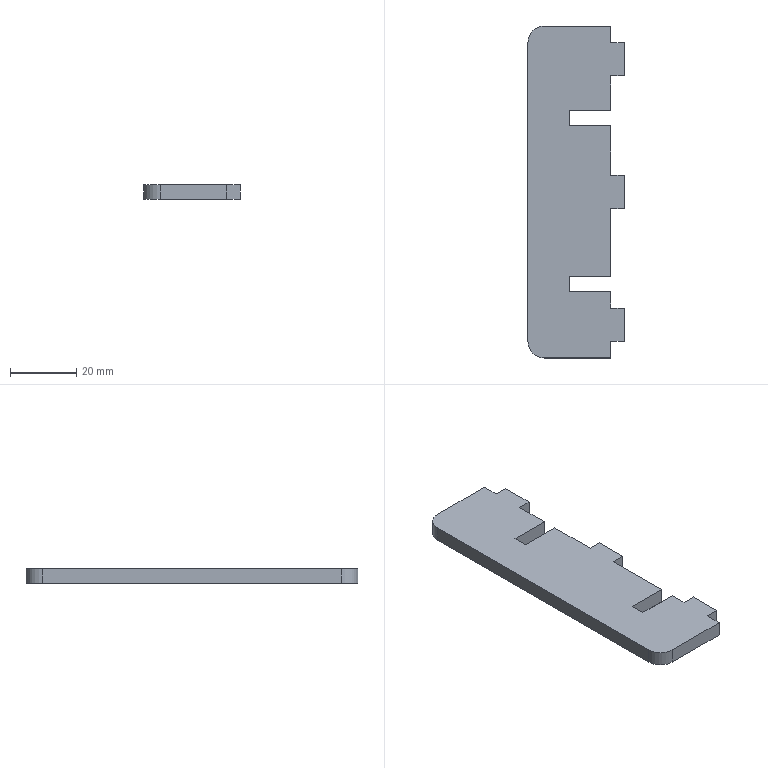Part | SolidWorks | features FlatPattern 1, SMBaseFlange 1, SheetMetal 1 | 1 solid | 28 faces | box 29 x 100 x 4.5 mm | volume 11235 mm3 | plane 26 | cylinder 2 | commonest cylinder face diameters 10 x2
STEP:
#1=CARTESIAN_POINT('',(115.747,10.575,0.));
#2=VERTEX_POINT('',#1);
#3=CARTESIAN_POINT('',(115.747,15.575,0.));
#4=VERTEX_POINT('',#3);
#5=CARTESIAN_POINT('',(115.747,15.575,0.));
#6=DIRECTION('',(0.,1.,0.));
#7=VECTOR('',#6,1000.);
#8=LINE('',#5,#7);
#9=EDGE_CURVE('',#2,#4,#8,.T.);
#10=ORIENTED_EDGE('',*,*,#9,.F.);
#11=CARTESIAN_POINT('',(115.747,10.575,-4.5));
#12=VERTEX_POINT('',#11);
#13=CARTESIAN_POINT('',(115.747,10.575,-4.5));
#14=DIRECTION('',(0.,0.,1.));
#15=VECTOR('',#14,1000.);
#16=LINE('',#13,#15);
#17=EDGE_CURVE('',#12,#2,#16,.T.);
#18=ORIENTED_EDGE('',*,*,#17,.F.);
#19=CARTESIAN_POINT('',(115.747,15.575,-4.5));
#20=VERTEX_POINT('',#19);
#21=CARTESIAN_POINT('',(115.747,15.575,-4.5));
#22=DIRECTION('',(0.,1.,0.));
#23=VECTOR('',#22,1000.);
#24=LINE('',#21,#23);
#25=EDGE_CURVE('',#12,#20,#24,.T.);
#26=ORIENTED_EDGE('',*,*,#25,.T.);
#27=CARTESIAN_POINT('',(115.747,15.575,-4.5));
#28=DIRECTION('',(0.,0.,1.));
#29=VECTOR('',#28,1000.);
#30=LINE('',#27,#29);
#31=EDGE_CURVE('',#20,#4,#30,.T.);
#32=ORIENTED_EDGE('',*,*,#31,.T.);
#33=EDGE_LOOP('',(#10,#18,#26,#32));
#34=FACE_OUTER_BOUND('',#33,.T.);
#35=CARTESIAN_POINT('',(115.747,15.575,-4.5));
#36=DIRECTION('',(1.,0.,0.));
#37=DIRECTION('',(0.,0.,-1.));
#38=AXIS2_PLACEMENT_3D('',#35,#36,#37);
#39=PLANE('',#38);
#40=ADVANCED_FACE('',(#34),#39,.T.);
#41=CARTESIAN_POINT('',(119.747,10.575,0.));
#42=VERTEX_POINT('',#41);
#43=CARTESIAN_POINT('',(115.747,10.575,0.));
#44=DIRECTION('',(-1.,0.,0.));
#45=VECTOR('',#44,1000.);
#46=LINE('',#43,#45);
#47=EDGE_CURVE('',#42,#2,#46,.T.);
#48=ORIENTED_EDGE('',*,*,#47,.F.);
#49=CARTESIAN_POINT('',(119.747,10.575,-4.5));
#50=VERTEX_POINT('',#49);
#51=CARTESIAN_POINT('',(119.747,10.575,-4.5));
#52=DIRECTION('',(0.,0.,1.));
#53=VECTOR('',#52,1000.);
#54=LINE('',#51,#53);
#55=EDGE_CURVE('',#50,#42,#54,.T.);
#56=ORIENTED_EDGE('',*,*,#55,.F.);
#57=CARTESIAN_POINT('',(115.747,10.575,-4.5));
#58=DIRECTION('',(-1.,0.,0.));
#59=VECTOR('',#58,1000.);
#60=LINE('',#57,#59);
#61=EDGE_CURVE('',#50,#12,#60,.T.);
#62=ORIENTED_EDGE('',*,*,#61,.T.);
#63=ORIENTED_EDGE('',*,*,#17,.T.);
#64=EDGE_LOOP('',(#48,#56,#62,#63));
#65=FACE_OUTER_BOUND('',#64,.T.);
#66=CARTESIAN_POINT('',(115.747,10.575,-4.5));
#67=DIRECTION('',(0.,1.,0.));
#68=DIRECTION('',(0.,0.,1.));
#69=AXIS2_PLACEMENT_3D('',#66,#67,#68);
#70=PLANE('',#69);
#71=ADVANCED_FACE('',(#65),#70,.T.);
#72=CARTESIAN_POINT('',(119.747,0.5749,0.));
#73=VERTEX_POINT('',#72);
#74=CARTESIAN_POINT('',(119.747,10.575,0.));
#75=DIRECTION('',(0.,1.,0.));
#76=VECTOR('',#75,1000.);
#77=LINE('',#74,#76);
#78=EDGE_CURVE('',#73,#42,#77,.T.);
#79=ORIENTED_EDGE('',*,*,#78,.F.);
#80=CARTESIAN_POINT('',(119.747,0.5749,-4.5));
#81=VERTEX_POINT('',#80);
#82=CARTESIAN_POINT('',(119.747,0.5749,-4.5));
#83=DIRECTION('',(0.,0.,1.));
#84=VECTOR('',#83,1000.);
#85=LINE('',#82,#84);
#86=EDGE_CURVE('',#81,#73,#85,.T.);
#87=ORIENTED_EDGE('',*,*,#86,.F.);
#88=CARTESIAN_POINT('',(119.747,10.575,-4.5));
#89=DIRECTION('',(0.,1.,0.));
#90=VECTOR('',#89,1000.);
#91=LINE('',#88,#90);
#92=EDGE_CURVE('',#81,#50,#91,.T.);
#93=ORIENTED_EDGE('',*,*,#92,.T.);
#94=ORIENTED_EDGE('',*,*,#55,.T.);
#95=EDGE_LOOP('',(#79,#87,#93,#94));
#96=FACE_OUTER_BOUND('',#95,.T.);
#97=CARTESIAN_POINT('',(119.747,10.575,-4.5));
#98=DIRECTION('',(1.,0.,0.));
#99=DIRECTION('',(0.,0.,-1.));
#100=AXIS2_PLACEMENT_3D('',#97,#98,#99);
#101=PLANE('',#100);
#102=ADVANCED_FACE('',(#96),#101,.T.);
#103=CARTESIAN_POINT('',(115.747,0.5749,0.));
#104=VERTEX_POINT('',#103);
#105=CARTESIAN_POINT('',(119.747,0.5749,0.));
#106=DIRECTION('',(1.,0.,0.));
#107=VECTOR('',#106,1000.);
#108=LINE('',#105,#107);
#109=EDGE_CURVE('',#104,#73,#108,.T.);
#110=ORIENTED_EDGE('',*,*,#109,.F.);
#111=CARTESIAN_POINT('',(115.747,0.5749,-4.5));
#112=VERTEX_POINT('',#111);
#113=CARTESIAN_POINT('',(115.747,0.5749,-4.5));
#114=DIRECTION('',(0.,0.,1.));
#115=VECTOR('',#114,1000.);
#116=LINE('',#113,#115);
#117=EDGE_CURVE('',#112,#104,#116,.T.);
#118=ORIENTED_EDGE('',*,*,#117,.F.);
#119=CARTESIAN_POINT('',(119.747,0.5749,-4.5));
#120=DIRECTION('',(1.,0.,0.));
#121=VECTOR('',#120,1000.);
#122=LINE('',#119,#121);
#123=EDGE_CURVE('',#112,#81,#122,.T.);
#124=ORIENTED_EDGE('',*,*,#123,.T.);
#125=ORIENTED_EDGE('',*,*,#86,.T.);
#126=EDGE_LOOP('',(#110,#118,#124,#125));
#127=FACE_OUTER_BOUND('',#126,.T.);
#128=CARTESIAN_POINT('',(119.747,0.5749,-4.5));
#129=DIRECTION('',(0.,-1.,0.));
#130=DIRECTION('',(1.,0.,0.));
#131=AXIS2_PLACEMENT_3D('',#128,#129,#130);
#132=PLANE('',#131);
#133=ADVANCED_FACE('',(#127),#132,.T.);
#134=CARTESIAN_POINT('',(115.747,-9.925,0.));
#135=VERTEX_POINT('',#134);
#136=CARTESIAN_POINT('',(115.747,0.5749,0.));
#137=DIRECTION('',(0.,1.,0.));
#138=VECTOR('',#137,1000.);
#139=LINE('',#136,#138);
#140=EDGE_CURVE('',#135,#104,#139,.T.);
#141=ORIENTED_EDGE('',*,*,#140,.F.);
#142=CARTESIAN_POINT('',(115.747,-9.925,-4.5));
#143=VERTEX_POINT('',#142);
#144=CARTESIAN_POINT('',(115.747,-9.925,-4.5));
#145=DIRECTION('',(0.,0.,1.));
#146=VECTOR('',#145,1000.);
#147=LINE('',#144,#146);
#148=EDGE_CURVE('',#143,#135,#147,.T.);
#149=ORIENTED_EDGE('',*,*,#148,.F.);
#150=CARTESIAN_POINT('',(115.747,0.5749,-4.5));
#151=DIRECTION('',(0.,1.,0.));
#152=VECTOR('',#151,1000.);
#153=LINE('',#150,#152);
#154=EDGE_CURVE('',#143,#112,#153,.T.);
#155=ORIENTED_EDGE('',*,*,#154,.T.);
#156=ORIENTED_EDGE('',*,*,#117,.T.);
#157=EDGE_LOOP('',(#141,#149,#155,#156));
#158=FACE_OUTER_BOUND('',#157,.T.);
#159=CARTESIAN_POINT('',(115.747,0.5749,-4.5));
#160=DIRECTION('',(1.,0.,0.));
#161=DIRECTION('',(0.,1.,0.));
#162=AXIS2_PLACEMENT_3D('',#159,#160,#161);
#163=PLANE('',#162);
#164=ADVANCED_FACE('',(#158),#163,.T.);
#165=CARTESIAN_POINT('',(103.247,-9.925,0.));
#166=VERTEX_POINT('',#165);
#167=CARTESIAN_POINT('',(115.747,-9.925,0.));
#168=DIRECTION('',(1.,0.,0.));
#169=VECTOR('',#168,1000.);
#170=LINE('',#167,#169);
#171=EDGE_CURVE('',#166,#135,#170,.T.);
#172=ORIENTED_EDGE('',*,*,#171,.F.);
#173=CARTESIAN_POINT('',(103.247,-9.925,-4.5));
#174=VERTEX_POINT('',#173);
#175=CARTESIAN_POINT('',(103.247,-9.925,-4.5));
#176=DIRECTION('',(0.,0.,1.));
#177=VECTOR('',#176,1000.);
#178=LINE('',#175,#177);
#179=EDGE_CURVE('',#174,#166,#178,.T.);
#180=ORIENTED_EDGE('',*,*,#179,.F.);
#181=CARTESIAN_POINT('',(115.747,-9.925,-4.5));
#182=DIRECTION('',(1.,0.,0.));
#183=VECTOR('',#182,1000.);
#184=LINE('',#181,#183);
#185=EDGE_CURVE('',#174,#143,#184,.T.);
#186=ORIENTED_EDGE('',*,*,#185,.T.);
#187=ORIENTED_EDGE('',*,*,#148,.T.);
#188=EDGE_LOOP('',(#172,#180,#186,#187));
#189=FACE_OUTER_BOUND('',#188,.T.);
#190=CARTESIAN_POINT('',(115.747,-9.925,-4.5));
#191=DIRECTION('',(0.,-1.,0.));
#192=DIRECTION('',(0.,0.,-1.));
#193=AXIS2_PLACEMENT_3D('',#190,#191,#192);
#194=PLANE('',#193);
#195=ADVANCED_FACE('',(#189),#194,.T.);
#196=CARTESIAN_POINT('',(103.247,-14.425,0.));
#197=VERTEX_POINT('',#196);
#198=CARTESIAN_POINT('',(103.247,-9.925,0.));
#199=DIRECTION('',(0.,1.,0.));
#200=VECTOR('',#199,1000.);
#201=LINE('',#198,#200);
#202=EDGE_CURVE('',#197,#166,#201,.T.);
#203=ORIENTED_EDGE('',*,*,#202,.F.);
#204=CARTESIAN_POINT('',(103.247,-14.425,-4.5));
#205=VERTEX_POINT('',#204);
#206=CARTESIAN_POINT('',(103.247,-14.425,-4.5));
#207=DIRECTION('',(0.,0.,1.));
#208=VECTOR('',#207,1000.);
#209=LINE('',#206,#208);
#210=EDGE_CURVE('',#205,#197,#209,.T.);
#211=ORIENTED_EDGE('',*,*,#210,.F.);
#212=CARTESIAN_POINT('',(103.247,-9.925,-4.5));
#213=DIRECTION('',(0.,1.,0.));
#214=VECTOR('',#213,1000.);
#215=LINE('',#212,#214);
#216=EDGE_CURVE('',#205,#174,#215,.T.);
#217=ORIENTED_EDGE('',*,*,#216,.T.);
#218=ORIENTED_EDGE('',*,*,#179,.T.);
#219=EDGE_LOOP('',(#203,#211,#217,#218));
#220=FACE_OUTER_BOUND('',#219,.T.);
#221=CARTESIAN_POINT('',(103.247,-9.925,-4.5));
#222=DIRECTION('',(1.,0.,0.));
#223=DIRECTION('',(0.,0.,-1.));
#224=AXIS2_PLACEMENT_3D('',#221,#222,#223);
#225=PLANE('',#224);
#226=ADVANCED_FACE('',(#220),#225,.T.);
#227=CARTESIAN_POINT('',(115.747,-14.425,0.));
#228=VERTEX_POINT('',#227);
#229=CARTESIAN_POINT('',(103.247,-14.425,0.));
#230=DIRECTION('',(-1.,0.,0.));
#231=VECTOR('',#230,1000.);
#232=LINE('',#229,#231);
#233=EDGE_CURVE('',#228,#197,#232,.T.);
#234=ORIENTED_EDGE('',*,*,#233,.F.);
#235=CARTESIAN_POINT('',(115.747,-14.425,-4.5));
#236=VERTEX_POINT('',#235);
#237=CARTESIAN_POINT('',(115.747,-14.425,-4.5));
#238=DIRECTION('',(0.,0.,1.));
#239=VECTOR('',#238,1000.);
#240=LINE('',#237,#239);
#241=EDGE_CURVE('',#236,#228,#240,.T.);
#242=ORIENTED_EDGE('',*,*,#241,.F.);
#243=CARTESIAN_POINT('',(103.247,-14.425,-4.5));
#244=DIRECTION('',(-1.,0.,0.));
#245=VECTOR('',#244,1000.);
#246=LINE('',#243,#245);
#247=EDGE_CURVE('',#236,#205,#246,.T.);
#248=ORIENTED_EDGE('',*,*,#247,.T.);
#249=ORIENTED_EDGE('',*,*,#210,.T.);
#250=EDGE_LOOP('',(#234,#242,#248,#249));
#251=FACE_OUTER_BOUND('',#250,.T.);
#252=CARTESIAN_POINT('',(103.247,-14.425,-4.5));
#253=DIRECTION('',(0.,1.,0.));
#254=DIRECTION('',(0.,0.,1.));
#255=AXIS2_PLACEMENT_3D('',#252,#253,#254);
#256=PLANE('',#255);
#257=ADVANCED_FACE('',(#251),#256,.T.);
#258=CARTESIAN_POINT('',(115.747,-29.425,0.));
#259=VERTEX_POINT('',#258);
#260=CARTESIAN_POINT('',(115.747,-14.425,0.));
#261=DIRECTION('',(0.,1.,0.));
#262=VECTOR('',#261,1000.);
#263=LINE('',#260,#262);
#264=EDGE_CURVE('',#259,#228,#263,.T.);
#265=ORIENTED_EDGE('',*,*,#264,.F.);
#266=CARTESIAN_POINT('',(115.747,-29.425,-4.5));
#267=VERTEX_POINT('',#266);
#268=CARTESIAN_POINT('',(115.747,-29.425,-4.5));
#269=DIRECTION('',(0.,0.,1.));
#270=VECTOR('',#269,1000.);
#271=LINE('',#268,#270);
#272=EDGE_CURVE('',#267,#259,#271,.T.);
#273=ORIENTED_EDGE('',*,*,#272,.F.);
#274=CARTESIAN_POINT('',(115.747,-14.425,-4.5));
#275=DIRECTION('',(0.,1.,0.));
#276=VECTOR('',#275,1000.);
#277=LINE('',#274,#276);
#278=EDGE_CURVE('',#267,#236,#277,.T.);
#279=ORIENTED_EDGE('',*,*,#278,.T.);
#280=ORIENTED_EDGE('',*,*,#241,.T.);
#281=EDGE_LOOP('',(#265,#273,#279,#280));
#282=FACE_OUTER_BOUND('',#281,.T.);
#283=CARTESIAN_POINT('',(115.747,-14.425,-4.5));
#284=DIRECTION('',(1.,0.,0.));
#285=DIRECTION('',(0.,1.,0.));
#286=AXIS2_PLACEMENT_3D('',#283,#284,#285);
#287=PLANE('',#286);
#288=ADVANCED_FACE('',(#282),#287,.T.);
#289=CARTESIAN_POINT('',(119.747,-29.425,0.));
#290=VERTEX_POINT('',#289);
#291=CARTESIAN_POINT('',(115.747,-29.425,0.));
#292=DIRECTION('',(-1.,0.,0.));
#293=VECTOR('',#292,1000.);
#294=LINE('',#291,#293);
#295=EDGE_CURVE('',#290,#259,#294,.T.);
#296=ORIENTED_EDGE('',*,*,#295,.F.);
#297=CARTESIAN_POINT('',(119.747,-29.425,-4.5));
#298=VERTEX_POINT('',#297);
#299=CARTESIAN_POINT('',(119.747,-29.425,-4.5));
#300=DIRECTION('',(0.,0.,1.));
#301=VECTOR('',#300,1000.);
#302=LINE('',#299,#301);
#303=EDGE_CURVE('',#298,#290,#302,.T.);
#304=ORIENTED_EDGE('',*,*,#303,.F.);
#305=CARTESIAN_POINT('',(115.747,-29.425,-4.5));
#306=DIRECTION('',(-1.,0.,0.));
#307=VECTOR('',#306,1000.);
#308=LINE('',#305,#307);
#309=EDGE_CURVE('',#298,#267,#308,.T.);
#310=ORIENTED_EDGE('',*,*,#309,.T.);
#311=ORIENTED_EDGE('',*,*,#272,.T.);
#312=EDGE_LOOP('',(#296,#304,#310,#311));
#313=FACE_OUTER_BOUND('',#312,.T.);
#314=CARTESIAN_POINT('',(115.747,-29.425,-4.5));
#315=DIRECTION('',(0.,1.,0.));
#316=DIRECTION('',(0.,0.,1.));
#317=AXIS2_PLACEMENT_3D('',#314,#315,#316);
#318=PLANE('',#317);
#319=ADVANCED_FACE('',(#313),#318,.T.);
#320=CARTESIAN_POINT('',(119.747,-39.425,0.));
#321=VERTEX_POINT('',#320);
#322=CARTESIAN_POINT('',(119.747,-29.425,0.));
#323=DIRECTION('',(0.,1.,0.));
#324=VECTOR('',#323,1000.);
#325=LINE('',#322,#324);
#326=EDGE_CURVE('',#321,#290,#325,.T.);
#327=ORIENTED_EDGE('',*,*,#326,.F.);
#328=CARTESIAN_POINT('',(119.747,-39.425,-4.5));
#329=VERTEX_POINT('',#328);
#330=CARTESIAN_POINT('',(119.747,-39.425,-4.5));
#331=DIRECTION('',(0.,0.,1.));
#332=VECTOR('',#331,1000.);
#333=LINE('',#330,#332);
#334=EDGE_CURVE('',#329,#321,#333,.T.);
#335=ORIENTED_EDGE('',*,*,#334,.F.);
#336=CARTESIAN_POINT('',(119.747,-29.425,-4.5));
#337=DIRECTION('',(0.,1.,0.));
#338=VECTOR('',#337,1000.);
#339=LINE('',#336,#338);
#340=EDGE_CURVE('',#329,#298,#339,.T.);
#341=ORIENTED_EDGE('',*,*,#340,.T.);
#342=ORIENTED_EDGE('',*,*,#303,.T.);
#343=EDGE_LOOP('',(#327,#335,#341,#342));
#344=FACE_OUTER_BOUND('',#343,.T.);
#345=CARTESIAN_POINT('',(119.747,-29.425,-4.5));
#346=DIRECTION('',(1.,0.,0.));
#347=DIRECTION('',(0.,0.,-1.));
#348=AXIS2_PLACEMENT_3D('',#345,#346,#347);
#349=PLANE('',#348);
#350=ADVANCED_FACE('',(#344),#349,.T.);
#351=CARTESIAN_POINT('',(115.747,-39.425,0.));
#352=VERTEX_POINT('',#351);
#353=CARTESIAN_POINT('',(119.747,-39.425,0.));
#354=DIRECTION('',(1.,0.,0.));
#355=VECTOR('',#354,1000.);
#356=LINE('',#353,#355);
#357=EDGE_CURVE('',#352,#321,#356,.T.);
#358=ORIENTED_EDGE('',*,*,#357,.F.);
#359=CARTESIAN_POINT('',(115.747,-39.425,-4.5));
#360=VERTEX_POINT('',#359);
#361=CARTESIAN_POINT('',(115.747,-39.425,-4.5));
#362=DIRECTION('',(0.,0.,1.));
#363=VECTOR('',#362,1000.);
#364=LINE('',#361,#363);
#365=EDGE_CURVE('',#360,#352,#364,.T.);
#366=ORIENTED_EDGE('',*,*,#365,.F.);
#367=CARTESIAN_POINT('',(119.747,-39.425,-4.5));
#368=DIRECTION('',(1.,0.,0.));
#369=VECTOR('',#368,1000.);
#370=LINE('',#367,#369);
#371=EDGE_CURVE('',#360,#329,#370,.T.);
#372=ORIENTED_EDGE('',*,*,#371,.T.);
#373=ORIENTED_EDGE('',*,*,#334,.T.);
#374=EDGE_LOOP('',(#358,#366,#372,#373));
#375=FACE_OUTER_BOUND('',#374,.T.);
#376=CARTESIAN_POINT('',(119.747,-39.425,-4.5));
#377=DIRECTION('',(0.,-1.,0.));
#378=DIRECTION('',(0.,0.,-1.));
#379=AXIS2_PLACEMENT_3D('',#376,#377,#378);
#380=PLANE('',#379);
#381=ADVANCED_FACE('',(#375),#380,.T.);
#382=CARTESIAN_POINT('',(115.747,-59.925,0.));
#383=VERTEX_POINT('',#382);
#384=CARTESIAN_POINT('',(115.747,-39.425,0.));
#385=DIRECTION('',(0.,1.,0.));
#386=VECTOR('',#385,1000.);
#387=LINE('',#384,#386);
#388=EDGE_CURVE('',#383,#352,#387,.T.);
#389=ORIENTED_EDGE('',*,*,#388,.F.);
#390=CARTESIAN_POINT('',(115.747,-59.925,-4.5));
#391=VERTEX_POINT('',#390);
#392=CARTESIAN_POINT('',(115.747,-59.925,-4.5));
#393=DIRECTION('',(0.,0.,1.));
#394=VECTOR('',#393,1000.);
#395=LINE('',#392,#394);
#396=EDGE_CURVE('',#391,#383,#395,.T.);
#397=ORIENTED_EDGE('',*,*,#396,.F.);
#398=CARTESIAN_POINT('',(115.747,-39.425,-4.5));
#399=DIRECTION('',(0.,1.,0.));
#400=VECTOR('',#399,1000.);
#401=LINE('',#398,#400);
#402=EDGE_CURVE('',#391,#360,#401,.T.);
#403=ORIENTED_EDGE('',*,*,#402,.T.);
#404=ORIENTED_EDGE('',*,*,#365,.T.);
#405=EDGE_LOOP('',(#389,#397,#403,#404));
#406=FACE_OUTER_BOUND('',#405,.T.);
#407=CARTESIAN_POINT('',(115.747,-39.425,-4.5));
#408=DIRECTION('',(1.,0.,0.));
#409=DIRECTION('',(0.,1.,0.));
#410=AXIS2_PLACEMENT_3D('',#407,#408,#409);
#411=PLANE('',#410);
#412=ADVANCED_FACE('',(#406),#411,.T.);
#413=CARTESIAN_POINT('',(103.247,-59.925,0.));
#414=VERTEX_POINT('',#413);
#415=CARTESIAN_POINT('',(115.747,-59.925,0.));
#416=DIRECTION('',(1.,0.,0.));
#417=VECTOR('',#416,1000.);
#418=LINE('',#415,#417);
#419=EDGE_CURVE('',#414,#383,#418,.T.);
#420=ORIENTED_EDGE('',*,*,#419,.F.);
#421=CARTESIAN_POINT('',(103.247,-59.925,-4.5));
#422=VERTEX_POINT('',#421);
#423=CARTESIAN_POINT('',(103.247,-59.925,-4.5));
#424=DIRECTION('',(0.,0.,1.));
#425=VECTOR('',#424,1000.);
#426=LINE('',#423,#425);
#427=EDGE_CURVE('',#422,#414,#426,.T.);
#428=ORIENTED_EDGE('',*,*,#427,.F.);
#429=CARTESIAN_POINT('',(115.747,-59.925,-4.5));
#430=DIRECTION('',(1.,0.,0.));
#431=VECTOR('',#430,1000.);
#432=LINE('',#429,#431);
#433=EDGE_CURVE('',#422,#391,#432,.T.);
#434=ORIENTED_EDGE('',*,*,#433,.T.);
#435=ORIENTED_EDGE('',*,*,#396,.T.);
#436=EDGE_LOOP('',(#420,#428,#434,#435));
#437=FACE_OUTER_BOUND('',#436,.T.);
#438=CARTESIAN_POINT('',(115.747,-59.925,-4.5));
#439=DIRECTION('',(0.,-1.,0.));
#440=DIRECTION('',(0.,0.,-1.));
#441=AXIS2_PLACEMENT_3D('',#438,#439,#440);
#442=PLANE('',#441);
#443=ADVANCED_FACE('',(#437),#442,.T.);
#444=CARTESIAN_POINT('',(103.247,-64.425,0.));
#445=VERTEX_POINT('',#444);
#446=CARTESIAN_POINT('',(103.247,-59.925,0.));
#447=DIRECTION('',(0.,1.,0.));
#448=VECTOR('',#447,1000.);
#449=LINE('',#446,#448);
#450=EDGE_CURVE('',#445,#414,#449,.T.);
#451=ORIENTED_EDGE('',*,*,#450,.F.);
#452=CARTESIAN_POINT('',(103.247,-64.425,-4.5));
#453=VERTEX_POINT('',#452);
#454=CARTESIAN_POINT('',(103.247,-64.425,-4.5));
#455=DIRECTION('',(0.,0.,1.));
#456=VECTOR('',#455,1000.);
#457=LINE('',#454,#456);
#458=EDGE_CURVE('',#453,#445,#457,.T.);
#459=ORIENTED_EDGE('',*,*,#458,.F.);
#460=CARTESIAN_POINT('',(103.247,-59.925,-4.5));
#461=DIRECTION('',(0.,1.,0.));
#462=VECTOR('',#461,1000.);
#463=LINE('',#460,#462);
#464=EDGE_CURVE('',#453,#422,#463,.T.);
#465=ORIENTED_EDGE('',*,*,#464,.T.);
#466=ORIENTED_EDGE('',*,*,#427,.T.);
#467=EDGE_LOOP('',(#451,#459,#465,#466));
#468=FACE_OUTER_BOUND('',#467,.T.);
#469=CARTESIAN_POINT('',(103.247,-59.925,-4.5));
#470=DIRECTION('',(1.,0.,0.));
#471=DIRECTION('',(0.,0.,-1.));
#472=AXIS2_PLACEMENT_3D('',#469,#470,#471);
#473=PLANE('',#472);
#474=ADVANCED_FACE('',(#468),#473,.T.);
#475=CARTESIAN_POINT('',(115.747,-64.425,0.));
#476=VERTEX_POINT('',#475);
#477=CARTESIAN_POINT('',(103.247,-64.425,0.));
#478=DIRECTION('',(-1.,0.,0.));
#479=VECTOR('',#478,1000.);
#480=LINE('',#477,#479);
#481=EDGE_CURVE('',#476,#445,#480,.T.);
#482=ORIENTED_EDGE('',*,*,#481,.F.);
#483=CARTESIAN_POINT('',(115.747,-64.425,-4.5));
#484=VERTEX_POINT('',#483);
#485=CARTESIAN_POINT('',(115.747,-64.425,-4.5));
#486=DIRECTION('',(0.,0.,1.));
#487=VECTOR('',#486,1000.);
#488=LINE('',#485,#487);
#489=EDGE_CURVE('',#484,#476,#488,.T.);
#490=ORIENTED_EDGE('',*,*,#489,.F.);
#491=CARTESIAN_POINT('',(103.247,-64.425,-4.5));
#492=DIRECTION('',(-1.,0.,0.));
#493=VECTOR('',#492,1000.);
#494=LINE('',#491,#493);
#495=EDGE_CURVE('',#484,#453,#494,.T.);
#496=ORIENTED_EDGE('',*,*,#495,.T.);
#497=ORIENTED_EDGE('',*,*,#458,.T.);
#498=EDGE_LOOP('',(#482,#490,#496,#497));
#499=FACE_OUTER_BOUND('',#498,.T.);
#500=CARTESIAN_POINT('',(103.247,-64.425,-4.5));
#501=DIRECTION('',(0.,1.,0.));
#502=DIRECTION('',(0.,0.,1.));
#503=AXIS2_PLACEMENT_3D('',#500,#501,#502);
#504=PLANE('',#503);
#505=ADVANCED_FACE('',(#499),#504,.T.);
#506=CARTESIAN_POINT('',(115.747,-69.425,0.));
#507=VERTEX_POINT('',#506);
#508=CARTESIAN_POINT('',(115.747,-64.425,0.));
#509=DIRECTION('',(0.,1.,0.));
#510=VECTOR('',#509,1000.);
#511=LINE('',#508,#510);
#512=EDGE_CURVE('',#507,#476,#511,.T.);
#513=ORIENTED_EDGE('',*,*,#512,.F.);
#514=CARTESIAN_POINT('',(115.747,-69.425,-4.5));
#515=VERTEX_POINT('',#514);
#516=CARTESIAN_POINT('',(115.747,-69.425,-4.5));
#517=DIRECTION('',(0.,0.,1.));
#518=VECTOR('',#517,1000.);
#519=LINE('',#516,#518);
#520=EDGE_CURVE('',#515,#507,#519,.T.);
#521=ORIENTED_EDGE('',*,*,#520,.F.);
#522=CARTESIAN_POINT('',(115.747,-64.425,-4.5));
#523=DIRECTION('',(0.,1.,0.));
#524=VECTOR('',#523,1000.);
#525=LINE('',#522,#524);
#526=EDGE_CURVE('',#515,#484,#525,.T.);
#527=ORIENTED_EDGE('',*,*,#526,.T.);
#528=ORIENTED_EDGE('',*,*,#489,.T.);
#529=EDGE_LOOP('',(#513,#521,#527,#528));
#530=FACE_OUTER_BOUND('',#529,.T.);
#531=CARTESIAN_POINT('',(115.747,-64.425,-4.5));
#532=DIRECTION('',(1.,0.,0.));
#533=DIRECTION('',(0.,0.,-1.));
#534=AXIS2_PLACEMENT_3D('',#531,#532,#533);
#535=PLANE('',#534);
#536=ADVANCED_FACE('',(#530),#535,.T.);
#537=CARTESIAN_POINT('',(119.747,-69.425,0.));
#538=VERTEX_POINT('',#537);
#539=CARTESIAN_POINT('',(119.747,-69.425,0.));
#540=DIRECTION('',(-1.,0.,0.));
#541=VECTOR('',#540,1000.);
#542=LINE('',#539,#541);
#543=EDGE_CURVE('',#538,#507,#542,.T.);
#544=ORIENTED_EDGE('',*,*,#543,.F.);
#545=CARTESIAN_POINT('',(119.747,-69.425,-4.5));
#546=VERTEX_POINT('',#545);
#547=CARTESIAN_POINT('',(119.747,-69.425,-4.5));
#548=DIRECTION('',(0.,0.,1.));
#549=VECTOR('',#548,1000.);
#550=LINE('',#547,#549);
#551=EDGE_CURVE('',#546,#538,#550,.T.);
#552=ORIENTED_EDGE('',*,*,#551,.F.);
#553=CARTESIAN_POINT('',(119.747,-69.425,-4.5));
#554=DIRECTION('',(-1.,0.,0.));
#555=VECTOR('',#554,1000.);
#556=LINE('',#553,#555);
#557=EDGE_CURVE('',#546,#515,#556,.T.);
#558=ORIENTED_EDGE('',*,*,#557,.T.);
#559=ORIENTED_EDGE('',*,*,#520,.T.);
#560=EDGE_LOOP('',(#544,#552,#558,#559));
#561=FACE_OUTER_BOUND('',#560,.T.);
#562=CARTESIAN_POINT('',(119.747,-69.425,-4.5));
#563=DIRECTION('',(0.,1.,0.));
#564=DIRECTION('',(0.,0.,1.));
#565=AXIS2_PLACEMENT_3D('',#562,#563,#564);
#566=PLANE('',#565);
#567=ADVANCED_FACE('',(#561),#566,.T.);
#568=CARTESIAN_POINT('',(119.747,-79.425,0.));
#569=VERTEX_POINT('',#568);
#570=CARTESIAN_POINT('',(119.747,-79.425,0.));
#571=DIRECTION('',(0.,1.,0.));
#572=VECTOR('',#571,1000.);
#573=LINE('',#570,#572);
#574=EDGE_CURVE('',#569,#538,#573,.T.);
#575=ORIENTED_EDGE('',*,*,#574,.F.);
#576=CARTESIAN_POINT('',(119.747,-79.425,-4.5));
#577=VERTEX_POINT('',#576);
#578=CARTESIAN_POINT('',(119.747,-79.425,-4.5));
#579=DIRECTION('',(0.,0.,1.));
#580=VECTOR('',#579,1000.);
#581=LINE('',#578,#580);
#582=EDGE_CURVE('',#577,#569,#581,.T.);
#583=ORIENTED_EDGE('',*,*,#582,.F.);
#584=CARTESIAN_POINT('',(119.747,-79.425,-4.5));
#585=DIRECTION('',(0.,1.,0.));
#586=VECTOR('',#585,1000.);
#587=LINE('',#584,#586);
#588=EDGE_CURVE('',#577,#546,#587,.T.);
#589=ORIENTED_EDGE('',*,*,#588,.T.);
#590=ORIENTED_EDGE('',*,*,#551,.T.);
#591=EDGE_LOOP('',(#575,#583,#589,#590));
#592=FACE_OUTER_BOUND('',#591,.T.);
#593=CARTESIAN_POINT('',(119.747,-79.425,-4.5));
#594=DIRECTION('',(1.,0.,0.));
#595=DIRECTION('',(0.,0.,-1.));
#596=AXIS2_PLACEMENT_3D('',#593,#594,#595);
#597=PLANE('',#596);
#598=ADVANCED_FACE('',(#592),#597,.T.);
#599=CARTESIAN_POINT('',(115.747,-79.425,0.));
#600=VERTEX_POINT('',#599);
#601=CARTESIAN_POINT('',(115.747,-79.425,0.));
#602=DIRECTION('',(1.,0.,0.));
#603=VECTOR('',#602,1000.);
#604=LINE('',#601,#603);
#605=EDGE_CURVE('',#600,#569,#604,.T.);
#606=ORIENTED_EDGE('',*,*,#605,.F.);
#607=CARTESIAN_POINT('',(115.747,-79.425,-4.5));
#608=VERTEX_POINT('',#607);
#609=CARTESIAN_POINT('',(115.747,-79.425,-4.5));
#610=DIRECTION('',(0.,0.,1.));
#611=VECTOR('',#610,1000.);
#612=LINE('',#609,#611);
#613=EDGE_CURVE('',#608,#600,#612,.T.);
#614=ORIENTED_EDGE('',*,*,#613,.F.);
#615=CARTESIAN_POINT('',(115.747,-79.425,-4.5));
#616=DIRECTION('',(1.,0.,0.));
#617=VECTOR('',#616,1000.);
#618=LINE('',#615,#617);
#619=EDGE_CURVE('',#608,#577,#618,.T.);
#620=ORIENTED_EDGE('',*,*,#619,.T.);
#621=ORIENTED_EDGE('',*,*,#582,.T.);
#622=EDGE_LOOP('',(#606,#614,#620,#621));
#623=FACE_OUTER_BOUND('',#622,.T.);
#624=CARTESIAN_POINT('',(115.747,-79.425,-4.5));
#625=DIRECTION('',(0.,-1.,0.));
#626=DIRECTION('',(0.,0.,-1.));
#627=AXIS2_PLACEMENT_3D('',#624,#625,#626);
#628=PLANE('',#627);
#629=ADVANCED_FACE('',(#623),#628,.T.);
#630=CARTESIAN_POINT('',(115.747,-84.425,0.));
#631=VERTEX_POINT('',#630);
#632=CARTESIAN_POINT('',(115.747,-79.425,0.));
#633=DIRECTION('',(0.,1.,0.));
#634=VECTOR('',#633,1000.);
#635=LINE('',#632,#634);
#636=EDGE_CURVE('',#631,#600,#635,.T.);
#637=ORIENTED_EDGE('',*,*,#636,.F.);
#638=CARTESIAN_POINT('',(115.747,-84.425,-4.5));
#639=VERTEX_POINT('',#638);
#640=CARTESIAN_POINT('',(115.747,-84.425,-4.5));
#641=DIRECTION('',(0.,0.,1.));
#642=VECTOR('',#641,1000.);
#643=LINE('',#640,#642);
#644=EDGE_CURVE('',#639,#631,#643,.T.);
#645=ORIENTED_EDGE('',*,*,#644,.F.);
#646=CARTESIAN_POINT('',(115.747,-79.425,-4.5));
#647=DIRECTION('',(0.,1.,0.));
#648=VECTOR('',#647,1000.);
#649=LINE('',#646,#648);
#650=EDGE_CURVE('',#639,#608,#649,.T.);
#651=ORIENTED_EDGE('',*,*,#650,.T.);
#652=ORIENTED_EDGE('',*,*,#613,.T.);
#653=EDGE_LOOP('',(#637,#645,#651,#652));
#654=FACE_OUTER_BOUND('',#653,.T.);
#655=CARTESIAN_POINT('',(115.747,-79.425,-4.5));
#656=DIRECTION('',(1.,0.,0.));
#657=DIRECTION('',(0.,0.,-1.));
#658=AXIS2_PLACEMENT_3D('',#655,#656,#657);
#659=PLANE('',#658);
#660=ADVANCED_FACE('',(#654),#659,.T.);
#661=CARTESIAN_POINT('',(95.747,-84.425,0.));
#662=VERTEX_POINT('',#661);
#663=CARTESIAN_POINT('',(115.747,-84.425,0.));
#664=DIRECTION('',(1.,0.,0.));
#665=VECTOR('',#664,1000.);
#666=LINE('',#663,#665);
#667=EDGE_CURVE('',#662,#631,#666,.T.);
#668=ORIENTED_EDGE('',*,*,#667,.F.);
#669=CARTESIAN_POINT('',(95.747,-84.425,-4.5));
#670=VERTEX_POINT('',#669);
#671=CARTESIAN_POINT('',(95.747,-84.425,-4.5));
#672=DIRECTION('',(0.,0.,1.));
#673=VECTOR('',#672,1000.);
#674=LINE('',#671,#673);
#675=EDGE_CURVE('',#670,#662,#674,.T.);
#676=ORIENTED_EDGE('',*,*,#675,.F.);
#677=CARTESIAN_POINT('',(115.747,-84.425,-4.5));
#678=DIRECTION('',(1.,0.,0.));
#679=VECTOR('',#678,1000.);
#680=LINE('',#677,#679);
#681=EDGE_CURVE('',#670,#639,#680,.T.);
#682=ORIENTED_EDGE('',*,*,#681,.T.);
#683=ORIENTED_EDGE('',*,*,#644,.T.);
#684=EDGE_LOOP('',(#668,#676,#682,#683));
#685=FACE_OUTER_BOUND('',#684,.T.);
#686=CARTESIAN_POINT('',(115.747,-84.425,-4.5));
#687=DIRECTION('',(0.,-1.,0.));
#688=DIRECTION('',(0.,0.,-1.));
#689=AXIS2_PLACEMENT_3D('',#686,#687,#688);
#690=PLANE('',#689);
#691=ADVANCED_FACE('',(#685),#690,.T.);
#692=CARTESIAN_POINT('',(90.747,-79.425,0.));
#693=VERTEX_POINT('',#692);
#694=CARTESIAN_POINT('',(95.747,-79.425,0.));
#695=DIRECTION('',(0.,0.,1.));
#696=DIRECTION('',(-1.,0.,0.));
#697=AXIS2_PLACEMENT_3D('',#694,#695,#696);
#698=CIRCLE('',#697,5.);
#699=EDGE_CURVE('',#693,#662,#698,.T.);
#700=ORIENTED_EDGE('',*,*,#699,.F.);
#701=CARTESIAN_POINT('',(90.747,-79.425,-4.5));
#702=VERTEX_POINT('',#701);
#703=CARTESIAN_POINT('',(90.747,-79.425,-4.5));
#704=DIRECTION('',(0.,0.,1.));
#705=VECTOR('',#704,1000.);
#706=LINE('',#703,#705);
#707=EDGE_CURVE('',#702,#693,#706,.T.);
#708=ORIENTED_EDGE('',*,*,#707,.F.);
#709=CARTESIAN_POINT('',(95.747,-79.425,-4.5));
#710=DIRECTION('',(0.,0.,1.));
#711=DIRECTION('',(-1.,0.,0.));
#712=AXIS2_PLACEMENT_3D('',#709,#710,#711);
#713=CIRCLE('',#712,5.);
#714=EDGE_CURVE('',#702,#670,#713,.T.);
#715=ORIENTED_EDGE('',*,*,#714,.T.);
#716=ORIENTED_EDGE('',*,*,#675,.T.);
#717=EDGE_LOOP('',(#700,#708,#715,#716));
#718=FACE_OUTER_BOUND('',#717,.T.);
#719=CARTESIAN_POINT('',(95.747,-79.425,-4.5));
#720=DIRECTION('',(0.,0.,1.));
#721=DIRECTION('',(1.,0.,0.));
#722=AXIS2_PLACEMENT_3D('',#719,#720,#721);
#723=CYLINDRICAL_SURFACE('',#722,5.);
#724=ADVANCED_FACE('',(#718),#723,.T.);
#725=CARTESIAN_POINT('',(90.747,10.575,0.));
#726=VERTEX_POINT('',#725);
#727=CARTESIAN_POINT('',(90.747,10.575,0.));
#728=DIRECTION('',(0.,-1.,0.));
#729=VECTOR('',#728,1000.);
#730=LINE('',#727,#729);
#731=EDGE_CURVE('',#726,#693,#730,.T.);
#732=ORIENTED_EDGE('',*,*,#731,.F.);
#733=CARTESIAN_POINT('',(90.747,10.575,-4.5));
#734=VERTEX_POINT('',#733);
#735=CARTESIAN_POINT('',(90.747,10.575,-4.5));
#736=DIRECTION('',(0.,0.,1.));
#737=VECTOR('',#736,1000.);
#738=LINE('',#735,#737);
#739=EDGE_CURVE('',#734,#726,#738,.T.);
#740=ORIENTED_EDGE('',*,*,#739,.F.);
#741=CARTESIAN_POINT('',(90.747,10.575,-4.5));
#742=DIRECTION('',(0.,-1.,0.));
#743=VECTOR('',#742,1000.);
#744=LINE('',#741,#743);
#745=EDGE_CURVE('',#734,#702,#744,.T.);
#746=ORIENTED_EDGE('',*,*,#745,.T.);
#747=ORIENTED_EDGE('',*,*,#707,.T.);
#748=EDGE_LOOP('',(#732,#740,#746,#747));
#749=FACE_OUTER_BOUND('',#748,.T.);
#750=CARTESIAN_POINT('',(90.747,10.575,-4.5));
#751=DIRECTION('',(-1.,0.,0.));
#752=DIRECTION('',(0.,-1.,0.));
#753=AXIS2_PLACEMENT_3D('',#750,#751,#752);
#754=PLANE('',#753);
#755=ADVANCED_FACE('',(#749),#754,.T.);
#756=CARTESIAN_POINT('',(95.747,15.575,0.));
#757=VERTEX_POINT('',#756);
#758=CARTESIAN_POINT('',(95.747,10.575,0.));
#759=DIRECTION('',(0.,0.,1.));
#760=DIRECTION('',(1.,0.,0.));
#761=AXIS2_PLACEMENT_3D('',#758,#759,#760);
#762=CIRCLE('',#761,5.);
#763=EDGE_CURVE('',#757,#726,#762,.T.);
#764=ORIENTED_EDGE('',*,*,#763,.F.);
#765=CARTESIAN_POINT('',(95.747,15.575,-4.5));
#766=VERTEX_POINT('',#765);
#767=CARTESIAN_POINT('',(95.747,15.575,-4.5));
#768=DIRECTION('',(0.,0.,1.));
#769=VECTOR('',#768,1000.);
#770=LINE('',#767,#769);
#771=EDGE_CURVE('',#766,#757,#770,.T.);
#772=ORIENTED_EDGE('',*,*,#771,.F.);
#773=CARTESIAN_POINT('',(95.747,10.575,-4.5));
#774=DIRECTION('',(0.,0.,1.));
#775=DIRECTION('',(1.,0.,0.));
#776=AXIS2_PLACEMENT_3D('',#773,#774,#775);
#777=CIRCLE('',#776,5.);
#778=EDGE_CURVE('',#766,#734,#777,.T.);
#779=ORIENTED_EDGE('',*,*,#778,.T.);
#780=ORIENTED_EDGE('',*,*,#739,.T.);
#781=EDGE_LOOP('',(#764,#772,#779,#780));
#782=FACE_OUTER_BOUND('',#781,.T.);
#783=CARTESIAN_POINT('',(95.747,10.575,-4.5));
#784=DIRECTION('',(0.,0.,1.));
#785=DIRECTION('',(1.,0.,0.));
#786=AXIS2_PLACEMENT_3D('',#783,#784,#785);
#787=CYLINDRICAL_SURFACE('',#786,5.);
#788=ADVANCED_FACE('',(#782),#787,.T.);
#789=CARTESIAN_POINT('',(115.747,15.575,0.));
#790=DIRECTION('',(-1.,0.,0.));
#791=VECTOR('',#790,1000.);
#792=LINE('',#789,#791);
#793=EDGE_CURVE('',#4,#757,#792,.T.);
#794=ORIENTED_EDGE('',*,*,#793,.F.);
#795=ORIENTED_EDGE('',*,*,#31,.F.);
#796=CARTESIAN_POINT('',(115.747,15.575,-4.5));
#797=DIRECTION('',(-1.,0.,0.));
#798=VECTOR('',#797,1000.);
#799=LINE('',#796,#798);
#800=EDGE_CURVE('',#20,#766,#799,.T.);
#801=ORIENTED_EDGE('',*,*,#800,.T.);
#802=ORIENTED_EDGE('',*,*,#771,.T.);
#803=EDGE_LOOP('',(#794,#795,#801,#802));
#804=FACE_OUTER_BOUND('',#803,.T.);
#805=CARTESIAN_POINT('',(115.747,15.575,-4.5));
#806=DIRECTION('',(0.,1.,0.));
#807=DIRECTION('',(-1.,0.,0.));
#808=AXIS2_PLACEMENT_3D('',#805,#806,#807);
#809=PLANE('',#808);
#810=ADVANCED_FACE('',(#804),#809,.T.);
#811=ORIENTED_EDGE('',*,*,#25,.F.);
#812=ORIENTED_EDGE('',*,*,#61,.F.);
#813=ORIENTED_EDGE('',*,*,#92,.F.);
#814=ORIENTED_EDGE('',*,*,#123,.F.);
#815=ORIENTED_EDGE('',*,*,#154,.F.);
#816=ORIENTED_EDGE('',*,*,#185,.F.);
#817=ORIENTED_EDGE('',*,*,#216,.F.);
#818=ORIENTED_EDGE('',*,*,#247,.F.);
#819=ORIENTED_EDGE('',*,*,#278,.F.);
#820=ORIENTED_EDGE('',*,*,#309,.F.);
#821=ORIENTED_EDGE('',*,*,#340,.F.);
#822=ORIENTED_EDGE('',*,*,#371,.F.);
#823=ORIENTED_EDGE('',*,*,#402,.F.);
#824=ORIENTED_EDGE('',*,*,#433,.F.);
#825=ORIENTED_EDGE('',*,*,#464,.F.);
#826=ORIENTED_EDGE('',*,*,#495,.F.);
#827=ORIENTED_EDGE('',*,*,#526,.F.);
#828=ORIENTED_EDGE('',*,*,#557,.F.);
#829=ORIENTED_EDGE('',*,*,#588,.F.);
#830=ORIENTED_EDGE('',*,*,#619,.F.);
#831=ORIENTED_EDGE('',*,*,#650,.F.);
#832=ORIENTED_EDGE('',*,*,#681,.F.);
#833=ORIENTED_EDGE('',*,*,#714,.F.);
#834=ORIENTED_EDGE('',*,*,#745,.F.);
#835=ORIENTED_EDGE('',*,*,#778,.F.);
#836=ORIENTED_EDGE('',*,*,#800,.F.);
#837=EDGE_LOOP('',(#811,#812,#813,#814,#815,#816,#817,#818,#819,#820,#821,#822,#823,#824,#825,#826,#827,#828,#829,#830,#831,#832,#833,#834,#835,#836));
#838=FACE_OUTER_BOUND('',#837,.T.);
#839=CARTESIAN_POINT('',(95.747,-79.425,-4.5));
#840=DIRECTION('',(0.,0.,-1.));
#841=DIRECTION('',(-1.,0.,0.));
#842=AXIS2_PLACEMENT_3D('',#839,#840,#841);
#843=PLANE('',#842);
#844=ADVANCED_FACE('',(#838),#843,.T.);
#845=ORIENTED_EDGE('',*,*,#9,.T.);
#846=ORIENTED_EDGE('',*,*,#793,.T.);
#847=ORIENTED_EDGE('',*,*,#763,.T.);
#848=ORIENTED_EDGE('',*,*,#731,.T.);
#849=ORIENTED_EDGE('',*,*,#699,.T.);
#850=ORIENTED_EDGE('',*,*,#667,.T.);
#851=ORIENTED_EDGE('',*,*,#636,.T.);
#852=ORIENTED_EDGE('',*,*,#605,.T.);
#853=ORIENTED_EDGE('',*,*,#574,.T.);
#854=ORIENTED_EDGE('',*,*,#543,.T.);
#855=ORIENTED_EDGE('',*,*,#512,.T.);
#856=ORIENTED_EDGE('',*,*,#481,.T.);
#857=ORIENTED_EDGE('',*,*,#450,.T.);
#858=ORIENTED_EDGE('',*,*,#419,.T.);
#859=ORIENTED_EDGE('',*,*,#388,.T.);
#860=ORIENTED_EDGE('',*,*,#357,.T.);
#861=ORIENTED_EDGE('',*,*,#326,.T.);
#862=ORIENTED_EDGE('',*,*,#295,.T.);
#863=ORIENTED_EDGE('',*,*,#264,.T.);
#864=ORIENTED_EDGE('',*,*,#233,.T.);
#865=ORIENTED_EDGE('',*,*,#202,.T.);
#866=ORIENTED_EDGE('',*,*,#171,.T.);
#867=ORIENTED_EDGE('',*,*,#140,.T.);
#868=ORIENTED_EDGE('',*,*,#109,.T.);
#869=ORIENTED_EDGE('',*,*,#78,.T.);
#870=ORIENTED_EDGE('',*,*,#47,.T.);
#871=EDGE_LOOP('',(#845,#846,#847,#848,#849,#850,#851,#852,#853,#854,#855,#856,#857,#858,#859,#860,#861,#862,#863,#864,#865,#866,#867,#868,#869,#870));
#872=FACE_OUTER_BOUND('',#871,.T.);
#873=CARTESIAN_POINT('',(95.747,-79.425,0.));
#874=DIRECTION('',(0.,0.,-1.));
#875=DIRECTION('',(-1.,0.,0.));
#876=AXIS2_PLACEMENT_3D('',#873,#874,#875);
#877=PLANE('',#876);
#878=ADVANCED_FACE('',(#872),#877,.F.);
#879=CLOSED_SHELL('',(#40,#71,#102,#133,#164,#195,#226,#257,#288,#319,#350,#381,#412,#443,#474,#505,#536,#567,#598,#629,#660,#691,#724,#755,#788,#810,#844,#878));
#880=MANIFOLD_SOLID_BREP('',#879);
#881=CARTESIAN_POINT('',(0.,0.,0.));
#882=DIRECTION('',(0.,0.,1.));
#883=DIRECTION('',(1.,0.,0.));
#884=AXIS2_PLACEMENT_3D('',#881,#882,#883);
#885=(LENGTH_UNIT()NAMED_UNIT(*)SI_UNIT(.MILLI.,.METRE.));
#886=UNCERTAINTY_MEASURE_WITH_UNIT(LENGTH_MEASURE(0.00001),#885,'','');
#887=(NAMED_UNIT(*)PLANE_ANGLE_UNIT()SI_UNIT($,.RADIAN.));
#888=(NAMED_UNIT(*)SI_UNIT($,.STERADIAN.)SOLID_ANGLE_UNIT());
#889=(GEOMETRIC_REPRESENTATION_CONTEXT(3)GLOBAL_UNCERTAINTY_ASSIGNED_CONTEXT((#886))GLOBAL_UNIT_ASSIGNED_CONTEXT((#885,#887,#888))REPRESENTATION_CONTEXT('',''));
#890=ADVANCED_BREP_SHAPE_REPRESENTATION('',(#880,#884),#889);